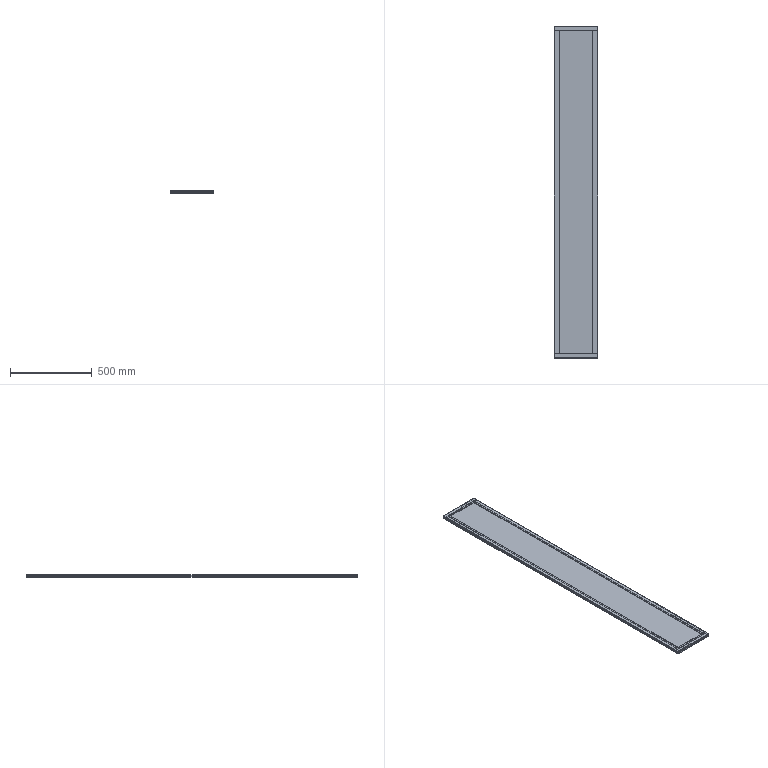Part | 5 solids | 167 faces | box 265 x 2036 x 18 mm | volume 5292562 mm3 | plane 98 | cylinder 69 | commonest cylinder face diameters 1.1 x24 3.6 x20 5.8 x20 1 x5